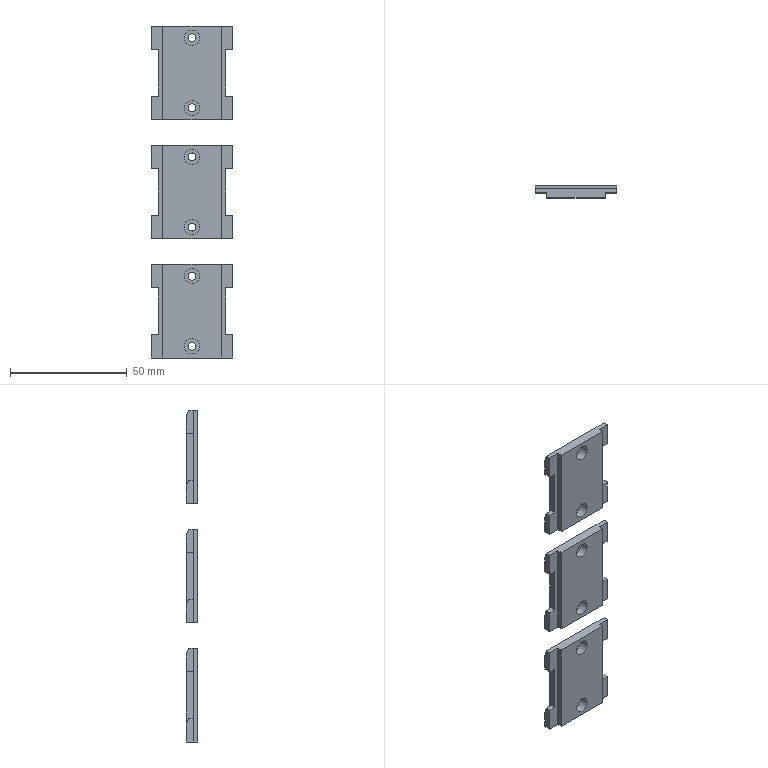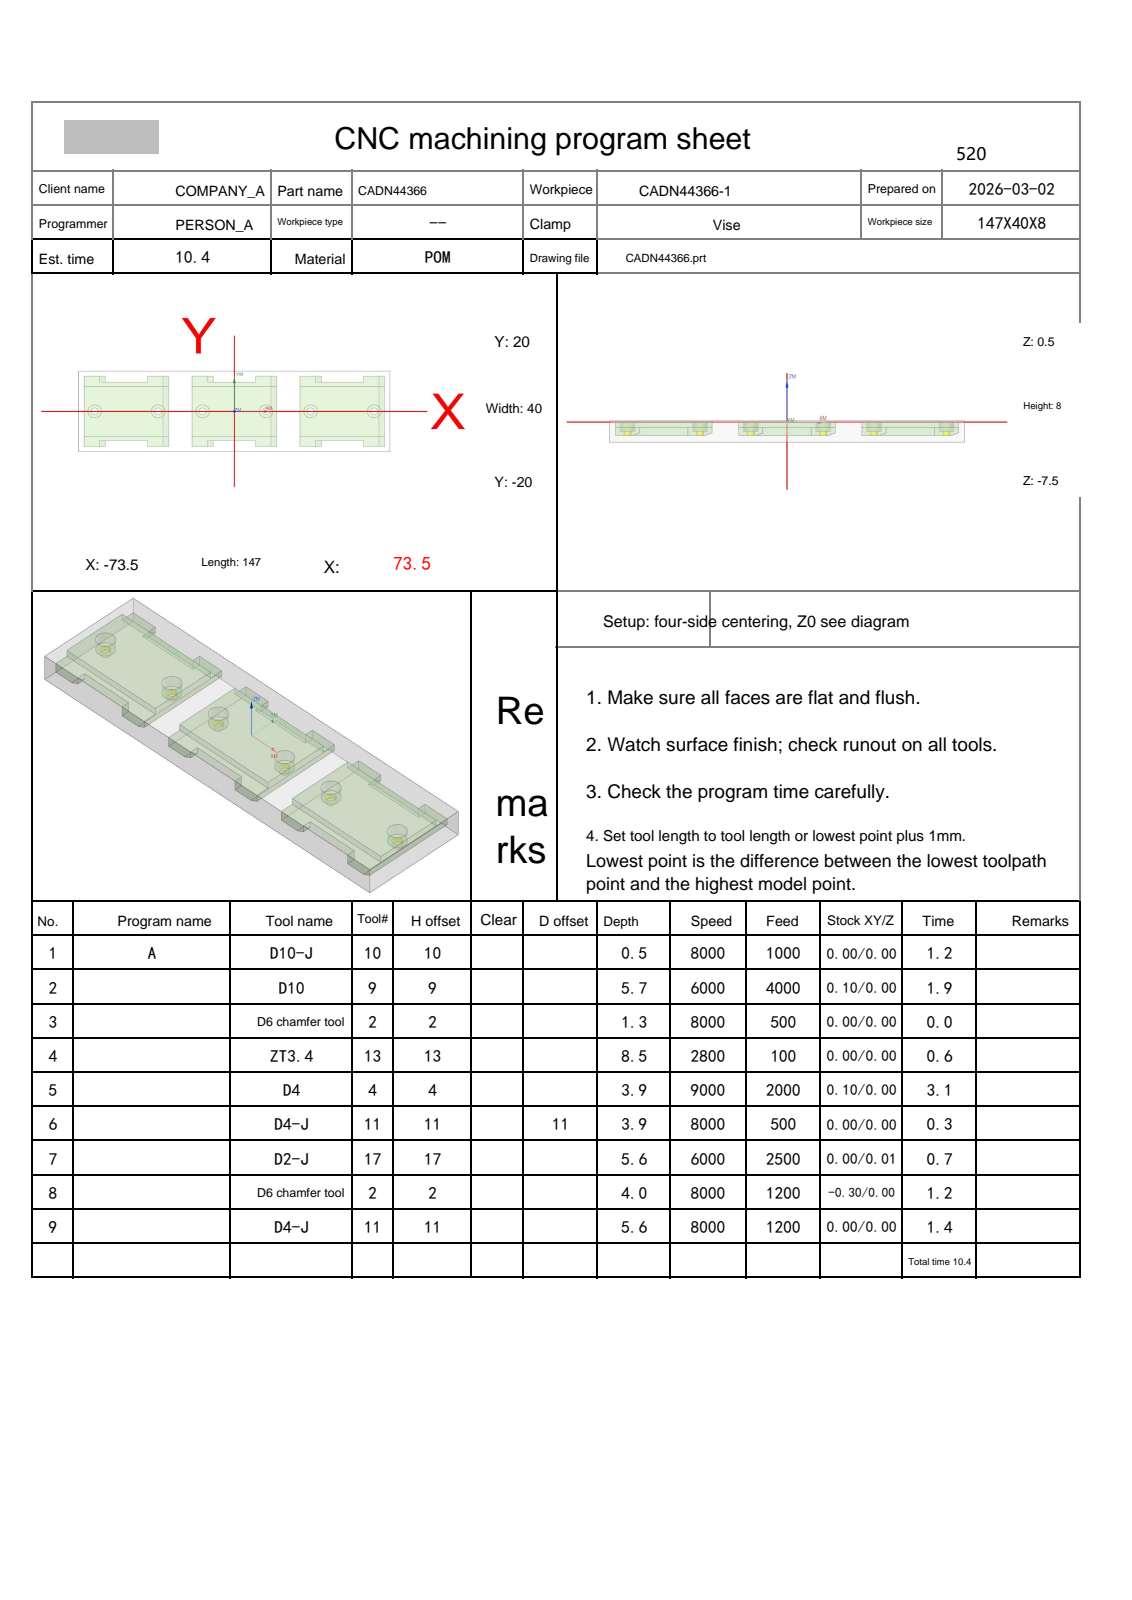NC program | NX | posted by the shop | part box 35 x 5 x 142 mm
Lines 1 to 1788 of 5584:
%
O0001
(Machine time: 11.93 MIN)
(===Total Tool:7===)
(T10=D10-J  D=10.  R=0.   D-  H10 Z=0.    )
(T9=D10     D=10.  R=0.   D-  H09 Z=-5.2  )
(T2=D6 chamfer tool   D=6.   R=0.   D-  H02 Z=-3.5  )
(T13=ZT3.4  D=3.4  DR_a=118 D-  H13 Z=-8.02 )
(T4=D4      D=4.   R=0.   D-  H04 Z=-3.4  )
(T11=D4-J   D=4.   R=0.   D11 H11 Z=-5.1  )
(T17=D2-J   D=2.   R=0.   D-  H17 Z=-5.1  )
G80 G90 G17 G49 G40
G91 G28 Z0
M01
N1 T10 M06
(D10-J  D=10. R=0. H=10 ce=0.00 di=0.00)
G00 G90 G54 X-88. Y.65 M03 S8000
G43 H10 Z30.
M08
Z2.
G01 Z0.0 F1000.
X-76. Y12.65
X-66.15 Y22.5
X-56.3
X-76. Y2.8
Y-7.05
X-46.45 Y22.5
X-36.6
X-76. Y-16.9
Y-22.5
X-71.75
X-26.75 Y22.5
X-16.9
X-61.9 Y-22.5
X-52.05
X-7.05 Y22.5
X2.8
X-42.2 Y-22.5
X-32.35
X12.65 Y22.5
X22.5
X-22.5 Y-22.5
X-12.65
X32.35 Y22.5
X42.2
X-2.8 Y-22.5
X7.05
X52.05 Y22.5
X61.9
X16.9 Y-22.5
X26.75
X71.75 Y22.5
X76.
Y16.9
X36.6 Y-22.5
X46.45
X76. Y7.05
Y-2.8
X56.3 Y-22.5
X66.15
X76. Y-12.65
X88. Y-.65
Z2.
G00 Z30.
G91 G28 Z0.0
M05
M09
G91 G28 Z0.0
M01
N2 T09 M06
(D10  D=10. R=0. H=09 ce=0.10 di=0.00)
G00 G90 G54 X76.1 Y0.0 M03 S6000
G43 H09 Z30.
M08
Z.5
G01 Y-17.5 Z.456 F4000.
G02 X71. Y-22.6 Z.435 I-5.1 J0.0
G01 X61. Z.41
G02 X56.352 Y-19.6 Z.395 I0.0 J5.1
G01 X45.648 Z.368
G02 X41. Y-22.6 Z.353 I-4.648 J2.1
G01 X31. Z.327
G02 X25.9 Y-17.5 Z.307 I0.0 J5.1
G01 Y17.5 Z.218
G02 X31. Y22.6 Z.198 I5.1 J0.0
G01 X41. Z.172
G02 X45.648 Y19.6 Z.157 I0.0 J-5.1
G01 X56.352 Z.13
G02 X61. Y22.6 Z.115 I4.648 J-2.1
G01 X71. Z.09
G02 X76.1 Y17.5 Z.069 I0.0 J-5.1
G01 Y-17.5 Z-.019
G02 X71. Y-22.6 Z-.04 I-5.1 J0.0
G01 X61. Z-.065
G02 X56.352 Y-19.6 Z-.08 I0.0 J5.1
G01 X45.648 Z-.107
G02 X41. Y-22.6 Z-.122 I-4.648 J2.1
G01 X31. Z-.148
G02 X25.9 Y-17.5 Z-.168 I0.0 J5.1
G01 Y17.5 Z-.257
G02 X31. Y22.6 Z-.277 I5.1 J0.0
G01 X41. Z-.303
G02 X45.648 Y19.6 Z-.318 I0.0 J-5.1
G01 X56.352 Z-.345
G02 X61. Y22.6 Z-.36 I4.648 J-2.1
G01 X71. Z-.385
G02 X76.1 Y17.5 Z-.406 I0.0 J-5.1
G01 Y-17.5 Z-.494
G02 X71. Y-22.6 Z-.515 I-5.1 J0.0
G01 X61. Z-.54
G02 X56.352 Y-19.6 Z-.555 I0.0 J5.1
G01 X45.648 Z-.582
G02 X41. Y-22.6 Z-.597 I-4.648 J2.1
G01 X31. Z-.623
G02 X25.9 Y-17.5 Z-.643 I0.0 J5.1
G01 Y17.5 Z-.732
G02 X31. Y22.6 Z-.752 I5.1 J0.0
G01 X41. Z-.778
G02 X45.648 Y19.6 Z-.793 I0.0 J-5.1
G01 X56.352 Z-.82
G02 X61. Y22.6 Z-.835 I4.648 J-2.1
G01 X71. Z-.86
G02 X76.1 Y17.5 Z-.881 I0.0 J-5.1
G01 Y-17.5 Z-.969
G02 X71. Y-22.6 Z-.99 I-5.1 J0.0
G01 X61. Z-1.015
G02 X56.352 Y-19.6 Z-1.03 I0.0 J5.1
G01 X45.648 Z-1.057
G02 X41. Y-22.6 Z-1.072 I-4.648 J2.1
G01 X31. Z-1.098
G02 X25.9 Y-17.5 Z-1.118 I0.0 J5.1
G01 Y17.5 Z-1.207
G02 X31. Y22.6 Z-1.227 I5.1 J0.0
G01 X41. Z-1.253
G02 X45.648 Y19.6 Z-1.268 I0.0 J-5.1
G01 X56.352 Z-1.295
G02 X61. Y22.6 Z-1.31 I4.648 J-2.1
G01 X71. Z-1.335
G02 X76.1 Y17.5 Z-1.356 I0.0 J-5.1
G01 Y-17.5 Z-1.444
G02 X71. Y-22.6 Z-1.465 I-5.1 J0.0
G01 X61. Z-1.49
G02 X56.352 Y-19.6 Z-1.505 I0.0 J5.1
G01 X45.648 Z-1.532
G02 X41. Y-22.6 Z-1.547 I-4.648 J2.1
G01 X31. Z-1.573
G02 X25.9 Y-17.5 Z-1.593 I0.0 J5.1
G01 Y17.5 Z-1.682
G02 X31. Y22.6 Z-1.702 I5.1 J0.0
G01 X41. Z-1.728
G02 X45.648 Y19.6 Z-1.743 I0.0 J-5.1
G01 X56.352 Z-1.77
G02 X61. Y22.6 Z-1.785 I4.648 J-2.1
G01 X71. Z-1.81
G02 X76.1 Y17.5 Z-1.831 I0.0 J-5.1
G01 Y-17.5 Z-1.919
G02 X71. Y-22.6 Z-1.94 I-5.1 J0.0
G01 X61. Z-1.965
G02 X56.352 Y-19.6 Z-1.98 I0.0 J5.1
G01 X45.648 Z-2.007
G02 X41. Y-22.6 Z-2.022 I-4.648 J2.1
G01 X31. Z-2.048
G02 X25.9 Y-17.5 Z-2.068 I0.0 J5.1
G01 Y17.5 Z-2.157
G02 X31. Y22.6 Z-2.177 I5.1 J0.0
G01 X41. Z-2.203
G02 X45.648 Y19.6 Z-2.218 I0.0 J-5.1
G01 X56.352 Z-2.245
G02 X61. Y22.6 Z-2.26 I4.648 J-2.1
G01 X71. Z-2.285
G02 X76.1 Y17.5 Z-2.306 I0.0 J-5.1
G01 Y-17.5 Z-2.394
G02 X71. Y-22.6 Z-2.415 I-5.1 J0.0
G01 X61. Z-2.44
G02 X56.352 Y-19.6 Z-2.455 I0.0 J5.1
G01 X45.648 Z-2.482
G02 X41. Y-22.6 Z-2.497 I-4.648 J2.1
G01 X31. Z-2.523
G02 X25.9 Y-17.5 Z-2.543 I0.0 J5.1
G01 Y17.5 Z-2.632
G02 X31. Y22.6 Z-2.652 I5.1 J0.0
G01 X41. Z-2.678
G02 X45.648 Y19.6 Z-2.693 I0.0 J-5.1
G01 X56.352 Z-2.72
G02 X61. Y22.6 Z-2.735 I4.648 J-2.1
G01 X71. Z-2.76
G02 X76.1 Y17.5 Z-2.781 I0.0 J-5.1
G01 Y-17.5 Z-2.869
G02 X71. Y-22.6 Z-2.89 I-5.1 J0.0
G01 X61. Z-2.915
G02 X56.352 Y-19.6 Z-2.93 I0.0 J5.1
G01 X45.648 Z-2.957
G02 X41. Y-22.6 Z-2.972 I-4.648 J2.1
G01 X31. Z-2.998
G02 X25.9 Y-17.5 Z-3.018 I0.0 J5.1
G01 Y17.5 Z-3.107
G02 X31. Y22.6 Z-3.127 I5.1 J0.0
G01 X41. Z-3.153
G02 X45.648 Y19.6 Z-3.168 I0.0 J-5.1
G01 X56.352 Z-3.195
G02 X61. Y22.6 Z-3.21 I4.648 J-2.1
G01 X71. Z-3.235
G02 X76.1 Y17.5 Z-3.256 I0.0 J-5.1
G01 Y-17.5 Z-3.344
G02 X71. Y-22.6 Z-3.365 I-5.1 J0.0
G01 X61. Z-3.39
G02 X56.352 Y-19.6 Z-3.405 I0.0 J5.1
G01 X45.648 Z-3.432
G02 X41. Y-22.6 Z-3.447 I-4.648 J2.1
G01 X31. Z-3.473
G02 X25.9 Y-17.5 Z-3.493 I0.0 J5.1
G01 Y17.5 Z-3.582
G02 X31. Y22.6 Z-3.602 I5.1 J0.0
G01 X41. Z-3.628
G02 X45.648 Y19.6 Z-3.643 I0.0 J-5.1
G01 X56.352 Z-3.67
G02 X61. Y22.6 Z-3.685 I4.648 J-2.1
G01 X71. Z-3.71
G02 X76.1 Y17.5 Z-3.731 I0.0 J-5.1
G01 Y-17.5 Z-3.819
G02 X71. Y-22.6 Z-3.84 I-5.1 J0.0
G01 X61. Z-3.865
G02 X56.352 Y-19.6 Z-3.88 I0.0 J5.1
G01 X45.648 Z-3.907
G02 X41. Y-22.6 Z-3.922 I-4.648 J2.1
G01 X31. Z-3.948
G02 X25.9 Y-17.5 Z-3.968 I0.0 J5.1
G01 Y17.5 Z-4.057
G02 X31. Y22.6 Z-4.077 I5.1 J0.0
G01 X41. Z-4.103
G02 X45.648 Y19.6 Z-4.118 I0.0 J-5.1
G01 X56.352 Z-4.145
G02 X61. Y22.6 Z-4.16 I4.648 J-2.1
G01 X71. Z-4.185
G02 X76.1 Y17.5 Z-4.206 I0.0 J-5.1
G01 Y-17.5 Z-4.294
G02 X71. Y-22.6 Z-4.315 I-5.1 J0.0
G01 X61. Z-4.34
G02 X56.352 Y-19.6 Z-4.355 I0.0 J5.1
G01 X45.648 Z-4.382
G02 X41. Y-22.6 Z-4.397 I-4.648 J2.1
G01 X31. Z-4.423
G02 X25.9 Y-17.5 Z-4.443 I0.0 J5.1
G01 Y17.5 Z-4.532
G02 X31. Y22.6 Z-4.552 I5.1 J0.0
G01 X41. Z-4.578
G02 X45.648 Y19.6 Z-4.593 I0.0 J-5.1
G01 X56.352 Z-4.62
G02 X61. Y22.6 Z-4.635 I4.648 J-2.1
G01 X71. Z-4.66
G02 X76.1 Y17.5 Z-4.681 I0.0 J-5.1
G01 Y-17.5 Z-4.769
G02 X71. Y-22.6 Z-4.79 I-5.1 J0.0
G01 X61. Z-4.815
G02 X56.352 Y-19.6 Z-4.83 I0.0 J5.1
G01 X45.648 Z-4.857
G02 X41. Y-22.6 Z-4.872 I-4.648 J2.1
G01 X31. Z-4.898
G02 X25.9 Y-17.5 Z-4.918 I0.0 J5.1
G01 Y17.5 Z-5.007
G02 X31. Y22.6 Z-5.027 I5.1 J0.0
G01 X41. Z-5.053
G02 X45.648 Y19.6 Z-5.068 I0.0 J-5.1
G01 X56.352 Z-5.095
G02 X61. Y22.6 Z-5.11 I4.648 J-2.1
G01 X71. Z-5.135
G02 X76.1 Y17.5 Z-5.156 I0.0 J-5.1
G01 Y0.0 Z-5.2
Y-17.5
G02 X71. Y-22.6 I-5.1 J0.0
G01 X61.
G02 X56.352 Y-19.6 I0.0 J5.1
G01 X45.648
G02 X41. Y-22.6 I-4.648 J2.1
G01 X31.
G02 X25.9 Y-17.5 I0.0 J5.1
G01 Y17.5
G02 X31. Y22.6 I5.1 J0.0
G01 X41.
G02 X45.648 Y19.6 I0.0 J-5.1
G01 X56.352
G02 X61. Y22.6 I4.648 J-2.1
G01 X71.
G02 X76.1 Y17.5 I0.0 J-5.1
G01 Y0.0
Y-.5
Z-4.2
G00 Z30.
X25.1 Y0.0
Z.5
G01 Y-17.5 Z.456
G02 X20. Y-22.6 Z.435 I-5.1 J0.0
G01 X10. Z.41
G02 X5.352 Y-19.6 Z.395 I0.0 J5.1
G01 X-5.352 Z.368
G02 X-10. Y-22.6 Z.353 I-4.648 J2.1
G01 X-20. Z.327
G02 X-25.1 Y-17.5 Z.307 I0.0 J5.1
G01 Y17.5 Z.218
G02 X-20. Y22.6 Z.198 I5.1 J0.0
G01 X-10. Z.172
G02 X-5.352 Y19.6 Z.157 I0.0 J-5.1
G01 X5.352 Z.13
G02 X10. Y22.6 Z.115 I4.648 J-2.1
G01 X20. Z.09
G02 X25.1 Y17.5 Z.069 I0.0 J-5.1
G01 Y-17.5 Z-.019
G02 X20. Y-22.6 Z-.04 I-5.1 J0.0
G01 X10. Z-.065
G02 X5.352 Y-19.6 Z-.08 I0.0 J5.1
G01 X-5.352 Z-.107
G02 X-10. Y-22.6 Z-.122 I-4.648 J2.1
G01 X-20. Z-.148
G02 X-25.1 Y-17.5 Z-.168 I0.0 J5.1
G01 Y17.5 Z-.257
G02 X-20. Y22.6 Z-.277 I5.1 J0.0
G01 X-10. Z-.303
G02 X-5.352 Y19.6 Z-.318 I0.0 J-5.1
G01 X5.352 Z-.345
G02 X10. Y22.6 Z-.36 I4.648 J-2.1
G01 X20. Z-.385
G02 X25.1 Y17.5 Z-.406 I0.0 J-5.1
G01 Y-17.5 Z-.494
G02 X20. Y-22.6 Z-.515 I-5.1 J0.0
G01 X10. Z-.54
G02 X5.352 Y-19.6 Z-.555 I0.0 J5.1
G01 X-5.352 Z-.582
G02 X-10. Y-22.6 Z-.597 I-4.648 J2.1
G01 X-20. Z-.623
G02 X-25.1 Y-17.5 Z-.643 I0.0 J5.1
G01 Y17.5 Z-.732
G02 X-20. Y22.6 Z-.752 I5.1 J0.0
G01 X-10. Z-.778
G02 X-5.352 Y19.6 Z-.793 I0.0 J-5.1
G01 X5.352 Z-.82
G02 X10. Y22.6 Z-.835 I4.648 J-2.1
G01 X20. Z-.86
G02 X25.1 Y17.5 Z-.881 I0.0 J-5.1
G01 Y-17.5 Z-.969
G02 X20. Y-22.6 Z-.99 I-5.1 J0.0
G01 X10. Z-1.015
G02 X5.352 Y-19.6 Z-1.03 I0.0 J5.1
G01 X-5.352 Z-1.057
G02 X-10. Y-22.6 Z-1.072 I-4.648 J2.1
G01 X-20. Z-1.098
G02 X-25.1 Y-17.5 Z-1.118 I0.0 J5.1
G01 Y17.5 Z-1.207
G02 X-20. Y22.6 Z-1.227 I5.1 J0.0
G01 X-10. Z-1.253
G02 X-5.352 Y19.6 Z-1.268 I0.0 J-5.1
G01 X5.352 Z-1.295
G02 X10. Y22.6 Z-1.31 I4.648 J-2.1
G01 X20. Z-1.335
G02 X25.1 Y17.5 Z-1.356 I0.0 J-5.1
G01 Y-17.5 Z-1.444
G02 X20. Y-22.6 Z-1.465 I-5.1 J0.0
G01 X10. Z-1.49
G02 X5.352 Y-19.6 Z-1.505 I0.0 J5.1
G01 X-5.352 Z-1.532
G02 X-10. Y-22.6 Z-1.547 I-4.648 J2.1
G01 X-20. Z-1.573
G02 X-25.1 Y-17.5 Z-1.593 I0.0 J5.1
G01 Y17.5 Z-1.682
G02 X-20. Y22.6 Z-1.702 I5.1 J0.0
G01 X-10. Z-1.728
G02 X-5.352 Y19.6 Z-1.743 I0.0 J-5.1
G01 X5.352 Z-1.77
G02 X10. Y22.6 Z-1.785 I4.648 J-2.1
G01 X20. Z-1.81
G02 X25.1 Y17.5 Z-1.831 I0.0 J-5.1
G01 Y-17.5 Z-1.919
G02 X20. Y-22.6 Z-1.94 I-5.1 J0.0
G01 X10. Z-1.965
G02 X5.352 Y-19.6 Z-1.98 I0.0 J5.1
G01 X-5.352 Z-2.007
G02 X-10. Y-22.6 Z-2.022 I-4.648 J2.1
G01 X-20. Z-2.048
G02 X-25.1 Y-17.5 Z-2.068 I0.0 J5.1
G01 Y17.5 Z-2.157
G02 X-20. Y22.6 Z-2.177 I5.1 J0.0
G01 X-10. Z-2.203
G02 X-5.352 Y19.6 Z-2.218 I0.0 J-5.1
G01 X5.352 Z-2.245
G02 X10. Y22.6 Z-2.26 I4.648 J-2.1
G01 X20. Z-2.285
G02 X25.1 Y17.5 Z-2.306 I0.0 J-5.1
G01 Y-17.5 Z-2.394
G02 X20. Y-22.6 Z-2.415 I-5.1 J0.0
G01 X10. Z-2.44
G02 X5.352 Y-19.6 Z-2.455 I0.0 J5.1
G01 X-5.352 Z-2.482
G02 X-10. Y-22.6 Z-2.497 I-4.648 J2.1
G01 X-20. Z-2.523
G02 X-25.1 Y-17.5 Z-2.543 I0.0 J5.1
G01 Y17.5 Z-2.632
G02 X-20. Y22.6 Z-2.652 I5.1 J0.0
G01 X-10. Z-2.678
G02 X-5.352 Y19.6 Z-2.693 I0.0 J-5.1
G01 X5.352 Z-2.72
G02 X10. Y22.6 Z-2.735 I4.648 J-2.1
G01 X20. Z-2.76
G02 X25.1 Y17.5 Z-2.781 I0.0 J-5.1
G01 Y-17.5 Z-2.869
G02 X20. Y-22.6 Z-2.89 I-5.1 J0.0
G01 X10. Z-2.915
G02 X5.352 Y-19.6 Z-2.93 I0.0 J5.1
G01 X-5.352 Z-2.957
G02 X-10. Y-22.6 Z-2.972 I-4.648 J2.1
G01 X-20. Z-2.998
G02 X-25.1 Y-17.5 Z-3.018 I0.0 J5.1
G01 Y17.5 Z-3.107
G02 X-20. Y22.6 Z-3.127 I5.1 J0.0
G01 X-10. Z-3.153
G02 X-5.352 Y19.6 Z-3.168 I0.0 J-5.1
G01 X5.352 Z-3.195
G02 X10. Y22.6 Z-3.21 I4.648 J-2.1
G01 X20. Z-3.235
G02 X25.1 Y17.5 Z-3.256 I0.0 J-5.1
G01 Y-17.5 Z-3.344
G02 X20. Y-22.6 Z-3.365 I-5.1 J0.0
G01 X10. Z-3.39
G02 X5.352 Y-19.6 Z-3.405 I0.0 J5.1
G01 X-5.352 Z-3.432
G02 X-10. Y-22.6 Z-3.447 I-4.648 J2.1
G01 X-20. Z-3.473
G02 X-25.1 Y-17.5 Z-3.493 I0.0 J5.1
G01 Y17.5 Z-3.582
G02 X-20. Y22.6 Z-3.602 I5.1 J0.0
G01 X-10. Z-3.628
G02 X-5.352 Y19.6 Z-3.643 I0.0 J-5.1
G01 X5.352 Z-3.67
G02 X10. Y22.6 Z-3.685 I4.648 J-2.1
G01 X20. Z-3.71
G02 X25.1 Y17.5 Z-3.731 I0.0 J-5.1
G01 Y-17.5 Z-3.819
G02 X20. Y-22.6 Z-3.84 I-5.1 J0.0
G01 X10. Z-3.865
G02 X5.352 Y-19.6 Z-3.88 I0.0 J5.1
G01 X-5.352 Z-3.907
G02 X-10. Y-22.6 Z-3.922 I-4.648 J2.1
G01 X-20. Z-3.948
G02 X-25.1 Y-17.5 Z-3.968 I0.0 J5.1
G01 Y17.5 Z-4.057
G02 X-20. Y22.6 Z-4.077 I5.1 J0.0
G01 X-10. Z-4.103
G02 X-5.352 Y19.6 Z-4.118 I0.0 J-5.1
G01 X5.352 Z-4.145
G02 X10. Y22.6 Z-4.16 I4.648 J-2.1
G01 X20. Z-4.185
G02 X25.1 Y17.5 Z-4.206 I0.0 J-5.1
G01 Y-17.5 Z-4.294
G02 X20. Y-22.6 Z-4.315 I-5.1 J0.0
G01 X10. Z-4.34
G02 X5.352 Y-19.6 Z-4.355 I0.0 J5.1
G01 X-5.352 Z-4.382
G02 X-10. Y-22.6 Z-4.397 I-4.648 J2.1
G01 X-20. Z-4.423
G02 X-25.1 Y-17.5 Z-4.443 I0.0 J5.1
G01 Y17.5 Z-4.532
G02 X-20. Y22.6 Z-4.552 I5.1 J0.0
G01 X-10. Z-4.578
G02 X-5.352 Y19.6 Z-4.593 I0.0 J-5.1
G01 X5.352 Z-4.62
G02 X10. Y22.6 Z-4.635 I4.648 J-2.1
G01 X20. Z-4.66
G02 X25.1 Y17.5 Z-4.681 I0.0 J-5.1
G01 Y-17.5 Z-4.769
G02 X20. Y-22.6 Z-4.79 I-5.1 J0.0
G01 X10. Z-4.815
G02 X5.352 Y-19.6 Z-4.83 I0.0 J5.1
G01 X-5.352 Z-4.857
G02 X-10. Y-22.6 Z-4.872 I-4.648 J2.1
G01 X-20. Z-4.898
G02 X-25.1 Y-17.5 Z-4.918 I0.0 J5.1
G01 Y17.5 Z-5.007
G02 X-20. Y22.6 Z-5.027 I5.1 J0.0
G01 X-10. Z-5.053
G02 X-5.352 Y19.6 Z-5.068 I0.0 J-5.1
G01 X5.352 Z-5.095
G02 X10. Y22.6 Z-5.11 I4.648 J-2.1
G01 X20. Z-5.135
G02 X25.1 Y17.5 Z-5.156 I0.0 J-5.1
G01 Y0.0 Z-5.2
Y-17.5
G02 X20. Y-22.6 I-5.1 J0.0
G01 X10.
G02 X5.352 Y-19.6 I0.0 J5.1
G01 X-5.352
G02 X-10. Y-22.6 I-4.648 J2.1
G01 X-20.
G02 X-25.1 Y-17.5 I0.0 J5.1
G01 Y17.5
G02 X-20. Y22.6 I5.1 J0.0
G01 X-10.
G02 X-5.352 Y19.6 I0.0 J-5.1
G01 X5.352
G02 X10. Y22.6 I4.648 J-2.1
G01 X20.
G02 X25.1 Y17.5 I0.0 J-5.1
G01 Y0.0
Y-.5
Z-4.2
G00 Z30.
X-76.1 Y0.0
Z.5
G01 Y17.5 Z.456
G02 X-71. Y22.6 Z.435 I5.1 J0.0
G01 X-61. Z.41
G02 X-56.352 Y19.6 Z.395 I0.0 J-5.1
G01 X-45.648 Z.368
G02 X-41. Y22.6 Z.353 I4.648 J-2.1
G01 X-31. Z.327
G02 X-25.9 Y17.5 Z.307 I0.0 J-5.1
G01 Y-17.5 Z.218
G02 X-31. Y-22.6 Z.198 I-5.1 J0.0
G01 X-41. Z.172
G02 X-45.648 Y-19.6 Z.157 I0.0 J5.1
G01 X-56.352 Z.13
G02 X-61. Y-22.6 Z.115 I-4.648 J2.1
G01 X-71. Z.09
G02 X-76.1 Y-17.5 Z.069 I0.0 J5.1
G01 Y17.5 Z-.019
G02 X-71. Y22.6 Z-.04 I5.1 J0.0
G01 X-61. Z-.065
G02 X-56.352 Y19.6 Z-.08 I0.0 J-5.1
G01 X-45.648 Z-.107
G02 X-41. Y22.6 Z-.122 I4.648 J-2.1
G01 X-31. Z-.148
G02 X-25.9 Y17.5 Z-.168 I0.0 J-5.1
G01 Y-17.5 Z-.257
G02 X-31. Y-22.6 Z-.277 I-5.1 J0.0
G01 X-41. Z-.303
G02 X-45.648 Y-19.6 Z-.318 I0.0 J5.1
G01 X-56.352 Z-.345
G02 X-61. Y-22.6 Z-.36 I-4.648 J2.1
G01 X-71. Z-.385
G02 X-76.1 Y-17.5 Z-.406 I0.0 J5.1
G01 Y17.5 Z-.494
G02 X-71. Y22.6 Z-.515 I5.1 J0.0
G01 X-61. Z-.54
G02 X-56.352 Y19.6 Z-.555 I0.0 J-5.1
G01 X-45.648 Z-.582
G02 X-41. Y22.6 Z-.597 I4.648 J-2.1
G01 X-31. Z-.623
G02 X-25.9 Y17.5 Z-.643 I0.0 J-5.1
G01 Y-17.5 Z-.732
G02 X-31. Y-22.6 Z-.752 I-5.1 J0.0
G01 X-41. Z-.778
G02 X-45.648 Y-19.6 Z-.793 I0.0 J5.1
G01 X-56.352 Z-.82
G02 X-61. Y-22.6 Z-.835 I-4.648 J2.1
G01 X-71. Z-.86
G02 X-76.1 Y-17.5 Z-.881 I0.0 J5.1
G01 Y17.5 Z-.969
G02 X-71. Y22.6 Z-.99 I5.1 J0.0
G01 X-61. Z-1.015
G02 X-56.352 Y19.6 Z-1.03 I0.0 J-5.1
G01 X-45.648 Z-1.057
G02 X-41. Y22.6 Z-1.072 I4.648 J-2.1
G01 X-31. Z-1.098
G02 X-25.9 Y17.5 Z-1.118 I0.0 J-5.1
G01 Y-17.5 Z-1.207
G02 X-31. Y-22.6 Z-1.227 I-5.1 J0.0
G01 X-41. Z-1.253
G02 X-45.648 Y-19.6 Z-1.268 I0.0 J5.1
G01 X-56.352 Z-1.295
G02 X-61. Y-22.6 Z-1.31 I-4.648 J2.1
G01 X-71. Z-1.335
G02 X-76.1 Y-17.5 Z-1.356 I0.0 J5.1
G01 Y17.5 Z-1.444
G02 X-71. Y22.6 Z-1.465 I5.1 J0.0
G01 X-61. Z-1.49
G02 X-56.352 Y19.6 Z-1.505 I0.0 J-5.1
G01 X-45.648 Z-1.532
G02 X-41. Y22.6 Z-1.547 I4.648 J-2.1
G01 X-31. Z-1.573
G02 X-25.9 Y17.5 Z-1.593 I0.0 J-5.1
G01 Y-17.5 Z-1.682
G02 X-31. Y-22.6 Z-1.702 I-5.1 J0.0
G01 X-41. Z-1.728
G02 X-45.648 Y-19.6 Z-1.743 I0.0 J5.1
G01 X-56.352 Z-1.77
G02 X-61. Y-22.6 Z-1.785 I-4.648 J2.1
G01 X-71. Z-1.81
G02 X-76.1 Y-17.5 Z-1.831 I0.0 J5.1
G01 Y17.5 Z-1.919
G02 X-71. Y22.6 Z-1.94 I5.1 J0.0
G01 X-61. Z-1.965
G02 X-56.352 Y19.6 Z-1.98 I0.0 J-5.1
G01 X-45.648 Z-2.007
G02 X-41. Y22.6 Z-2.022 I4.648 J-2.1
G01 X-31. Z-2.048
G02 X-25.9 Y17.5 Z-2.068 I0.0 J-5.1
G01 Y-17.5 Z-2.157
G02 X-31. Y-22.6 Z-2.177 I-5.1 J0.0
G01 X-41. Z-2.203
G02 X-45.648 Y-19.6 Z-2.218 I0.0 J5.1
G01 X-56.352 Z-2.245
G02 X-61. Y-22.6 Z-2.26 I-4.648 J2.1
G01 X-71. Z-2.285
G02 X-76.1 Y-17.5 Z-2.306 I0.0 J5.1
G01 Y17.5 Z-2.394
G02 X-71. Y22.6 Z-2.415 I5.1 J0.0
G01 X-61. Z-2.44
G02 X-56.352 Y19.6 Z-2.455 I0.0 J-5.1
G01 X-45.648 Z-2.482
G02 X-41. Y22.6 Z-2.497 I4.648 J-2.1
G01 X-31. Z-2.523
G02 X-25.9 Y17.5 Z-2.543 I0.0 J-5.1
G01 Y-17.5 Z-2.632
G02 X-31. Y-22.6 Z-2.652 I-5.1 J0.0
G01 X-41. Z-2.678
G02 X-45.648 Y-19.6 Z-2.693 I0.0 J5.1
G01 X-56.352 Z-2.72
G02 X-61. Y-22.6 Z-2.735 I-4.648 J2.1
G01 X-71. Z-2.76
G02 X-76.1 Y-17.5 Z-2.781 I0.0 J5.1
G01 Y17.5 Z-2.869
G02 X-71. Y22.6 Z-2.89 I5.1 J0.0
G01 X-61. Z-2.915
G02 X-56.352 Y19.6 Z-2.93 I0.0 J-5.1
G01 X-45.648 Z-2.957
G02 X-41. Y22.6 Z-2.972 I4.648 J-2.1
G01 X-31. Z-2.998
G02 X-25.9 Y17.5 Z-3.018 I0.0 J-5.1
G01 Y-17.5 Z-3.107
G02 X-31. Y-22.6 Z-3.127 I-5.1 J0.0
G01 X-41. Z-3.153
G02 X-45.648 Y-19.6 Z-3.168 I0.0 J5.1
G01 X-56.352 Z-3.195
G02 X-61. Y-22.6 Z-3.21 I-4.648 J2.1
G01 X-71. Z-3.235
G02 X-76.1 Y-17.5 Z-3.256 I0.0 J5.1
G01 Y17.5 Z-3.344
G02 X-71. Y22.6 Z-3.365 I5.1 J0.0
G01 X-61. Z-3.39
G02 X-56.352 Y19.6 Z-3.405 I0.0 J-5.1
G01 X-45.648 Z-3.432
G02 X-41. Y22.6 Z-3.447 I4.648 J-2.1
G01 X-31. Z-3.473
G02 X-25.9 Y17.5 Z-3.493 I0.0 J-5.1
G01 Y-17.5 Z-3.582
G02 X-31. Y-22.6 Z-3.602 I-5.1 J0.0
G01 X-41. Z-3.628
G02 X-45.648 Y-19.6 Z-3.643 I0.0 J5.1
G01 X-56.352 Z-3.67
G02 X-61. Y-22.6 Z-3.685 I-4.648 J2.1
G01 X-71. Z-3.71
G02 X-76.1 Y-17.5 Z-3.731 I0.0 J5.1
G01 Y17.5 Z-3.819
G02 X-71. Y22.6 Z-3.84 I5.1 J0.0
G01 X-61. Z-3.865
G02 X-56.352 Y19.6 Z-3.88 I0.0 J-5.1
G01 X-45.648 Z-3.907
G02 X-41. Y22.6 Z-3.922 I4.648 J-2.1
G01 X-31. Z-3.948
G02 X-25.9 Y17.5 Z-3.968 I0.0 J-5.1
G01 Y-17.5 Z-4.057
G02 X-31. Y-22.6 Z-4.077 I-5.1 J0.0
G01 X-41. Z-4.103
G02 X-45.648 Y-19.6 Z-4.118 I0.0 J5.1
G01 X-56.352 Z-4.145
G02 X-61. Y-22.6 Z-4.16 I-4.648 J2.1
G01 X-71. Z-4.185
G02 X-76.1 Y-17.5 Z-4.206 I0.0 J5.1
G01 Y17.5 Z-4.294
G02 X-71. Y22.6 Z-4.315 I5.1 J0.0
G01 X-61. Z-4.34
G02 X-56.352 Y19.6 Z-4.355 I0.0 J-5.1
G01 X-45.648 Z-4.382
G02 X-41. Y22.6 Z-4.397 I4.648 J-2.1
G01 X-31. Z-4.423
G02 X-25.9 Y17.5 Z-4.443 I0.0 J-5.1
G01 Y-17.5 Z-4.532
G02 X-31. Y-22.6 Z-4.552 I-5.1 J0.0
G01 X-41. Z-4.578
G02 X-45.648 Y-19.6 Z-4.593 I0.0 J5.1
G01 X-56.352 Z-4.62
G02 X-61. Y-22.6 Z-4.635 I-4.648 J2.1
G01 X-71. Z-4.66
G02 X-76.1 Y-17.5 Z-4.681 I0.0 J5.1
G01 Y17.5 Z-4.769
G02 X-71. Y22.6 Z-4.79 I5.1 J0.0
G01 X-61. Z-4.815
G02 X-56.352 Y19.6 Z-4.83 I0.0 J-5.1
G01 X-45.648 Z-4.857
G02 X-41. Y22.6 Z-4.872 I4.648 J-2.1
G01 X-31. Z-4.898
G02 X-25.9 Y17.5 Z-4.918 I0.0 J-5.1
G01 Y-17.5 Z-5.007
G02 X-31. Y-22.6 Z-5.027 I-5.1 J0.0
G01 X-41. Z-5.053
G02 X-45.648 Y-19.6 Z-5.068 I0.0 J5.1
G01 X-56.352 Z-5.095
G02 X-61. Y-22.6 Z-5.11 I-4.648 J2.1
G01 X-71. Z-5.135
G02 X-76.1 Y-17.5 Z-5.156 I0.0 J5.1
G01 Y0.0 Z-5.2
Y17.5
G02 X-71. Y22.6 I5.1 J0.0
G01 X-61.
G02 X-56.352 Y19.6 I0.0 J-5.1
G01 X-45.648
G02 X-41. Y22.6 I4.648 J-2.1
G01 X-31.
G02 X-25.9 Y17.5 I0.0 J-5.1
G01 Y-17.5
G02 X-31. Y-22.6 I-5.1 J0.0
G01 X-41.
G02 X-45.648 Y-19.6 I0.0 J5.1
G01 X-56.352
G02 X-61. Y-22.6 I-4.648 J2.1
G01 X-71.
G02 X-76.1 Y-17.5 I0.0 J5.1
G01 Y0.0
Y.5
Z-4.2
G00 Z30.
G91 G28 Z0.0
M05
M09
G91 G28 Z0.0
M01
N3 T02 M06
(D6 chamfer tool  D=6. R=0. H=02 ce=0.00 di=0.00)
G00 G90 G54 X-66. Y0.0 M03 S8000
G43 H02 Z30.
M08
G98 G81 X-66. Y0.0 Z-.8 R1. F500.
X-36.
X-15.
X15.
X36.
X66.
G80
G00 Z30.
G91 G28 Z0.0
M05
M09
G91 G28 Z0.0
M01
N4 T13 M06
(ZT3.4 D=3.4 DR_a=118 H=13)
G00 G90 G54 X-66. Y0.0 M03 S2800
G43 H13 Z30.
M08
G98 G83 X-66. Y0.0 Z-8.021 R1. F100. Q2.
X-36.
X-15.
X15.
X36.
X66.
G80
G00 Z30.
G91 G28 Z0.0
M05
M09
G91 G28 Z0.0
M01
N5 T04 M06
(D4  D=4. R=0. H=04 ce=0.10 di=0.10)
G00 G90 G54 X51. Y19.5 M03 S9000
G43 H04 Z30.
M08
Z.263
G01 Z-.238 F2000.
Y14.9
X41.4
Y17.9
X30.6
Y14.6
X71.4
Y17.9
X60.6
Y14.9
X51.
X50.5
Z.263
G00 Z.5
X51. Y19.5
Z.025
G01 Z-.475
Y14.9
X41.4
Y17.9
X30.6
Y14.6
X71.4
Y17.9
X60.6
Y14.9
X51.
X50.5
Z.025
G00 Z.263
X51. Y19.5
Z-.213
G01 Z-.713
Y14.9
X41.4
Y17.9
X30.6
Y14.6
X71.4
Y17.9
X60.6
Y14.9
X51.
X50.5
Z-.213
G00 Z.025
X51. Y19.5
Z-.45
G01 Z-.95
Y14.9
X41.4
Y17.9
X30.6
Y14.6
X71.4
Y17.9
X60.6
Y14.9
X51.
X50.5
Z-.45
G00 Z-.213
X51. Y19.5
Z-.688
G01 Z-1.188
Y14.9
X41.4
Y17.9
X30.6
Y14.6
X71.4
Y17.9
X60.6
Y14.9
X51.
X50.5
Z-.688
G00 Z-.45
X51. Y19.5
Z-.925
G01 Z-1.425
Y14.9
X41.4
Y17.9
X30.6
Y14.6
X71.4
Y17.9
X60.6
Y14.9
X51.
X50.5
Z-.925
G00 Z-.688
X51. Y19.5
Z-1.163
G01 Z-1.663
Y14.9
X41.4
Y17.9
X30.6
Y14.6
X71.4
Y17.9
X60.6
Y14.9
X51.
X50.5
Z-1.163
G00 Z-.925
X51. Y19.5
Z-1.4
G01 Z-1.9
Y14.9
X41.4
Y17.9
X30.6
Y14.6
X71.4
Y17.9
X60.6
Y14.9
X51.
X50.5
Z-1.4
G00 Z30.
X51. Y-19.5
Z.263
G01 Z-.238
Y-14.9
X60.6
Y-17.9
X71.4
Y-14.6
X30.6
Y-17.9
X41.4
Y-14.9
X51.
X51.5
Z.263
G00 Z.5
X51. Y-19.5
Z.025
G01 Z-.475
Y-14.9
X60.6
Y-17.9
X71.4
Y-14.6
X30.6
Y-17.9
X41.4
Y-14.9
X51.
X51.5
Z.025
G00 Z.263
X51. Y-19.5
Z-.213
G01 Z-.713
Y-14.9
X60.6
Y-17.9
X71.4
Y-14.6
X30.6
Y-17.9
X41.4
Y-14.9
X51.
X51.5
Z-.213
G00 Z.025
X51. Y-19.5
Z-.45
G01 Z-.95
Y-14.9
X60.6
Y-17.9
X71.4
Y-14.6
X30.6
Y-17.9
X41.4
Y-14.9
X51.
X51.5
Z-.45
G00 Z-.213
X51. Y-19.5
Z-.688
G01 Z-1.188
Y-14.9
X60.6
Y-17.9
X71.4
Y-14.6
X30.6
Y-17.9
X41.4
Y-14.9
X51.
X51.5
Z-.688
G00 Z-.45
X51. Y-19.5
Z-.925
G01 Z-1.425
Y-14.9
X60.6
Y-17.9
X71.4
Y-14.6
X30.6
Y-17.9
X41.4
Y-14.9
X51.
X51.5
Z-.925
G00 Z-.688
X51. Y-19.5
Z-1.163
G01 Z-1.663
Y-14.9
X60.6
Y-17.9
X71.4
Y-14.6
X30.6
Y-17.9
X41.4
Y-14.9
X51.
X51.5
Z-1.163
G00 Z-.925
X51. Y-19.5
Z-1.4
G01 Z-1.9
Y-14.9
X60.6
Y-17.9
X71.4
Y-14.6
X30.6
Y-17.9
X41.4
Y-14.9
X51.
X51.5
Z-1.4
G00 Z30.
X0.0 Y-19.5
Z.263
G01 Z-.238
Y-14.9
X9.6
Y-17.9
X20.4
Y-14.6
X-20.4
Y-17.9
X-9.6
Y-14.9
X0.0
X.5
Z.263
G00 Z.5
X0.0 Y-19.5
Z.025
G01 Z-.475
Y-14.9
X9.6
Y-17.9
X20.4
Y-14.6
X-20.4
Y-17.9
X-9.6
Y-14.9
X0.0
X.5
Z.025
G00 Z.263
X0.0 Y-19.5
Z-.213
G01 Z-.713
Y-14.9
X9.6
Y-17.9
X20.4
Y-14.6
X-20.4
Y-17.9
X-9.6
Y-14.9
X0.0
X.5
Z-.213
G00 Z.025
X0.0 Y-19.5
Z-.45
G01 Z-.95
Y-14.9
X9.6
Y-17.9
X20.4
Y-14.6
X-20.4
Y-17.9
X-9.6
Y-14.9
X0.0
X.5
Z-.45
G00 Z-.213
X0.0 Y-19.5
Z-.688
G01 Z-1.188
Y-14.9
X9.6
Y-17.9
X20.4
Y-14.6
X-20.4
Y-17.9
X-9.6
Y-14.9
X0.0
X.5
Z-.688
G00 Z-.45
X0.0 Y-19.5
Z-.925
G01 Z-1.425
Y-14.9
X9.6
Y-17.9
X20.4
Y-14.6
X-20.4
Y-17.9
X-9.6
Y-14.9
X0.0
X.5
Z-.925
G00 Z-.688
X0.0 Y-19.5
Z-1.163
G01 Z-1.663
Y-14.9
X9.6
Y-17.9
X20.4
Y-14.6
X-20.4
Y-17.9
X-9.6
Y-14.9
X0.0
X.5
Z-1.163
G00 Z-.925
X0.0 Y-19.5
Z-1.4
G01 Z-1.9
Y-14.9
X9.6
Y-17.9
X20.4
Y-14.6
X-20.4
Y-17.9
X-9.6
Y-14.9
X0.0
X.5
Z-1.4
G00 Z30.
X0.0 Y19.5
Z.263
G01 Z-.238
Y14.9
X-9.6
Y17.9
X-20.4
Y14.6
X20.4
Y17.9
X9.6
Y14.9
X0.0
X-.5
Z.263
G00 Z.5
X0.0 Y19.5
Z.025
G01 Z-.475
Y14.9
X-9.6
Y17.9
X-20.4
Y14.6
X20.4
Y17.9
X9.6
Y14.9
X0.0
X-.5
Z.025
G00 Z.263
X0.0 Y19.5
Z-.213
G01 Z-.713
Y14.9
X-9.6
Y17.9
X-20.4
Y14.6
X20.4
Y17.9
X9.6
Y14.9
X0.0
X-.5
Z-.213
G00 Z.025
X0.0 Y19.5
Z-.45
G01 Z-.95
Y14.9
X-9.6
Y17.9
X-20.4
Y14.6
X20.4
Y17.9
X9.6
Y14.9
X0.0
X-.5
Z-.45
G00 Z-.213
X0.0 Y19.5
Z-.688
G01 Z-1.188
Y14.9
X-9.6
Y17.9
X-20.4
Y14.6
X20.4
Y17.9
X9.6
Y14.9
X0.0
X-.5
Z-.688
G00 Z-.45
X0.0 Y19.5
Z-.925
G01 Z-1.425
Y14.9
X-9.6
Y17.9
X-20.4
Y14.6
X20.4
Y17.9
X9.6
Y14.9
X0.0
X-.5
Z-.925
G00 Z-.688
X0.0 Y19.5
Z-1.163
G01 Z-1.663
Y14.9
X-9.6
Y17.9
X-20.4
Y14.6
X20.4
Y17.9
X9.6
Y14.9
X0.0
X-.5
Z-1.163
G00 Z-.925
X0.0 Y19.5
Z-1.4
G01 Z-1.9
Y14.9
X-9.6
Y17.9
X-20.4
Y14.6
X20.4
Y17.9
X9.6
Y14.9
X0.0
X-.5
Z-1.4
G00 Z30.
X-51. Y19.5
Z.263
G01 Z-.238
Y14.9
X-60.6
Y17.9
X-71.4
Y14.6
X-30.6
Y17.9
X-41.4
Y14.9
X-51.
X-51.5
Z.263
G00 Z.5
X-51. Y19.5
Z.025
G01 Z-.475
Y14.9
X-60.6
Y17.9
X-71.4
Y14.6
X-30.6
Y17.9
X-41.4
Y14.9
X-51.
X-51.5
Z.025
G00 Z.263
X-51. Y19.5
Z-.213
G01 Z-.713
Y14.9
X-60.6
Y17.9
X-71.4
Y14.6
X-30.6
Y17.9
X-41.4
Y14.9
X-51.
X-51.5
Z-.213
G00 Z.025
X-51. Y19.5
Z-.45
G01 Z-.95
Y14.9
X-60.6
Y17.9
X-71.4
Y14.6
X-30.6
Y17.9
X-41.4
Y14.9
X-51.
X-51.5
Z-.45
G00 Z-.213
X-51. Y19.5
Z-.688
G01 Z-1.188
Y14.9
X-60.6
Y17.9
X-71.4
Y14.6
X-30.6
Y17.9
X-41.4
Y14.9
X-51.
X-51.5
Z-.688
G00 Z-.45
X-51. Y19.5
Z-.925
G01 Z-1.425
Y14.9
X-60.6
Y17.9
X-71.4
Y14.6
X-30.6
Y17.9
X-41.4
Y14.9
X-51.
X-51.5
Z-.925
G00 Z-.688
X-51. Y19.5
Z-1.163
G01 Z-1.663
Y14.9
X-60.6
Y17.9
X-71.4
Y14.6
X-30.6
Y17.9
X-41.4
Y14.9
X-51.
X-51.5
Z-1.163
G00 Z-.925
X-51. Y19.5
Z-1.4
G01 Z-1.9
Y14.9
X-60.6
Y17.9
X-71.4
Y14.6
X-30.6
Y17.9
X-41.4
Y14.9
X-51.
X-51.5
Z-1.4
G00 Z30.
X-51. Y-19.5
Z.263
G01 Z-.238
Y-14.9
X-41.4
Y-17.9
X-30.6
Y-14.6
X-71.4
Y-17.9
X-60.6
Y-14.9
X-51.
X-50.5
Z.263
G00 Z.5
X-51. Y-19.5
Z.025
G01 Z-.475
Y-14.9
X-41.4
Y-17.9
X-30.6
Y-14.6
X-71.4
Y-17.9
X-60.6
Y-14.9
X-51.
X-50.5
Z.025
G00 Z.263
X-51. Y-19.5
Z-.213
G01 Z-.713
Y-14.9
X-41.4
Y-17.9
X-30.6
Y-14.6
X-71.4
Y-17.9
X-60.6
Y-14.9
X-51.
X-50.5
Z-.213
G00 Z.025
X-51. Y-19.5
Z-.45
G01 Z-.95
Y-14.9
X-41.4
Y-17.9
X-30.6
Y-14.6
X-71.4
Y-17.9
X-60.6
Y-14.9
X-51.
X-50.5
Z-.45
G00 Z-.213
X-51. Y-19.5
Z-.688
G01 Z-1.188
Y-14.9
X-41.4
Y-17.9
X-30.6
Y-14.6
X-71.4
Y-17.9
X-60.6
Y-14.9
X-51.
X-50.5
Z-.688
G00 Z-.45
X-51. Y-19.5
Z-.925
G01 Z-1.425
Y-14.9
X-41.4
Y-17.9
X-30.6
Y-14.6
X-71.4
Y-17.9
X-60.6
Y-14.9
X-51.
X-50.5
Z-.925
G00 Z-.688
X-51. Y-19.5
Z-1.163
G01 Z-1.663
Y-14.9
X-41.4
Y-17.9
X-30.6
Y-14.6
X-71.4
Y-17.9
X-60.6
Y-14.9
X-51.
X-50.5
Z-1.163
G00 Z-.925
X-51. Y-19.5
Z-1.4
G01 Z-1.9
Y-14.9
X-41.4
Y-17.9
X-30.6
Y-14.6
X-71.4
Y-17.9
X-60.6
Y-14.9
X-51.
X-50.5
Z-1.4
G00 Z30.
G00 G90 X-66. Y0.0 M03 S8000
Z30.
Z.5
G03 X-66.575 Y-.575 I0.0 J-.575 F1200.
X-66. Y-1.15 I.575 J0.0
X-66. Y-1.15 Z.2 I0.0 J1.15
X-66. Y-1.15 Z-.1 I0.0 J1.15
X-66. Y-1.15 Z-.4 I0.0 J1.15
X-66. Y-1.15 Z-.7 I0.0 J1.15
X-66. Y-1.15 Z-1. I0.0 J1.15
X-66. Y-1.15 Z-1.3 I0.0 J1.15
X-66. Y-1.15 Z-1.6 I0.0 J1.15
X-66. Y-1.15 Z-1.9 I0.0 J1.15
X-66. Y-1.15 Z-2.2 I0.0 J1.15
X-66. Y-1.15 Z-2.5 I0.0 J1.15
X-66. Y-1.15 Z-2.8 I0.0 J1.15
X-66. Y-1.15 Z-3.1 I0.0 J1.15
X-66. Y-1.15 Z-3.4 I0.0 J1.15
X-64.85 Y0.0 I0.0 J1.15
X-66. Y1.15 I-1.15 J0.0
X-67.15 Y0.0 I0.0 J-1.15
X-66. Y-1.15 I1.15 J0.0
X-65.425 Y-.575 I0.0 J.575
X-66. Y0.0 I-.575 J0.0
G00 Z30.
X-36.
Z.5
G03 X-36.575 Y-.575 I0.0 J-.575
X-36. Y-1.15 I.575 J0.0
X-36. Y-1.15 Z.2 I0.0 J1.15
X-36. Y-1.15 Z-.1 I0.0 J1.15
X-36. Y-1.15 Z-.4 I0.0 J1.15
X-36. Y-1.15 Z-.7 I0.0 J1.15
X-36. Y-1.15 Z-1. I0.0 J1.15
X-36. Y-1.15 Z-1.3 I0.0 J1.15
X-36. Y-1.15 Z-1.6 I0.0 J1.15
X-36. Y-1.15 Z-1.9 I0.0 J1.15
X-36. Y-1.15 Z-2.2 I0.0 J1.15
X-36. Y-1.15 Z-2.5 I0.0 J1.15
X-36. Y-1.15 Z-2.8 I0.0 J1.15
X-36. Y-1.15 Z-3.1 I0.0 J1.15
X-36. Y-1.15 Z-3.4 I0.0 J1.15
X-34.85 Y0.0 I0.0 J1.15
X-36. Y1.15 I-1.15 J0.0
X-37.15 Y0.0 I0.0 J-1.15
X-36. Y-1.15 I1.15 J0.0
X-35.425 Y-.575 I0.0 J.575
X-36. Y0.0 I-.575 J0.0
G00 Z30.
X-15.
Z.5
G03 X-15.575 Y-.575 I0.0 J-.575
X-15. Y-1.15 I.575 J0.0
X-15. Y-1.15 Z.2 I0.0 J1.15
X-15. Y-1.15 Z-.1 I0.0 J1.15
X-15. Y-1.15 Z-.4 I0.0 J1.15
X-15. Y-1.15 Z-.7 I0.0 J1.15
X-15. Y-1.15 Z-1. I0.0 J1.15
X-15. Y-1.15 Z-1.3 I0.0 J1.15
X-15. Y-1.15 Z-1.6 I0.0 J1.15
X-15. Y-1.15 Z-1.9 I0.0 J1.15
X-15. Y-1.15 Z-2.2 I0.0 J1.15
X-15. Y-1.15 Z-2.5 I0.0 J1.15
X-15. Y-1.15 Z-2.8 I0.0 J1.15
X-15. Y-1.15 Z-3.1 I0.0 J1.15
X-15. Y-1.15 Z-3.4 I0.0 J1.15
X-13.85 Y0.0 I0.0 J1.15
X-15. Y1.15 I-1.15 J0.0
X-16.15 Y0.0 I0.0 J-1.15
X-15. Y-1.15 I1.15 J0.0
X-14.425 Y-.575 I0.0 J.575
X-15. Y0.0 I-.575 J0.0
G00 Z30.
X15.
Z.5
G03 X14.425 Y-.575 I0.0 J-.575
X15. Y-1.15 I.575 J0.0
X15. Y-1.15 Z.2 I0.0 J1.15
X15. Y-1.15 Z-.1 I0.0 J1.15
X15. Y-1.15 Z-.4 I0.0 J1.15
X15. Y-1.15 Z-.7 I0.0 J1.15
X15. Y-1.15 Z-1. I0.0 J1.15
X15. Y-1.15 Z-1.3 I0.0 J1.15
X15. Y-1.15 Z-1.6 I0.0 J1.15
X15. Y-1.15 Z-1.9 I0.0 J1.15
X15. Y-1.15 Z-2.2 I0.0 J1.15
X15. Y-1.15 Z-2.5 I0.0 J1.15
X15. Y-1.15 Z-2.8 I0.0 J1.15
X15. Y-1.15 Z-3.1 I0.0 J1.15
X15. Y-1.15 Z-3.4 I0.0 J1.15
X16.15 Y0.0 I0.0 J1.15
X15. Y1.15 I-1.15 J0.0
X13.85 Y0.0 I0.0 J-1.15
X15. Y-1.15 I1.15 J0.0
X15.575 Y-.575 I0.0 J.575
X15. Y0.0 I-.575 J0.0
G00 Z30.
X36.
Z.5
G03 X35.425 Y-.575 I0.0 J-.575
X36. Y-1.15 I.575 J0.0
X36. Y-1.15 Z.2 I0.0 J1.15
X36. Y-1.15 Z-.1 I0.0 J1.15
X36. Y-1.15 Z-.4 I0.0 J1.15
X36. Y-1.15 Z-.7 I0.0 J1.15
X36. Y-1.15 Z-1. I0.0 J1.15
X36. Y-1.15 Z-1.3 I0.0 J1.15
X36. Y-1.15 Z-1.6 I0.0 J1.15
X36. Y-1.15 Z-1.9 I0.0 J1.15
X36. Y-1.15 Z-2.2 I0.0 J1.15
X36. Y-1.15 Z-2.5 I0.0 J1.15
X36. Y-1.15 Z-2.8 I0.0 J1.15
X36. Y-1.15 Z-3.1 I0.0 J1.15
X36. Y-1.15 Z-3.4 I0.0 J1.15
X37.15 Y0.0 I0.0 J1.15
X36. Y1.15 I-1.15 J0.0
X34.85 Y0.0 I0.0 J-1.15
X36. Y-1.15 I1.15 J0.0
X36.575 Y-.575 I0.0 J.575
X36. Y0.0 I-.575 J0.0
G00 Z30.
X66.
Z.5
G03 X65.425 Y-.575 I0.0 J-.575
X66. Y-1.15 I.575 J0.0
X66. Y-1.15 Z.2 I0.0 J1.15
X66. Y-1.15 Z-.1 I0.0 J1.15
X66. Y-1.15 Z-.4 I0.0 J1.15
X66. Y-1.15 Z-.7 I0.0 J1.15
X66. Y-1.15 Z-1. I0.0 J1.15
X66. Y-1.15 Z-1.3 I0.0 J1.15
X66. Y-1.15 Z-1.6 I0.0 J1.15
X66. Y-1.15 Z-1.9 I0.0 J1.15
X66. Y-1.15 Z-2.2 I0.0 J1.15
X66. Y-1.15 Z-2.5 I0.0 J1.15
X66. Y-1.15 Z-2.8 I0.0 J1.15
X66. Y-1.15 Z-3.1 I0.0 J1.15
X66. Y-1.15 Z-3.4 I0.0 J1.15
X67.15 Y0.0 I0.0 J1.15
X66. Y1.15 I-1.15 J0.0
X64.85 Y0.0 I0.0 J-1.15
X66. Y-1.15 I1.15 J0.0
X66.575 Y-.575 I0.0 J.575
X66. Y0.0 I-.575 J0.0
G00 Z30.
G91 G28 Z0.0
M05
M09
G91 G28 Z0.0
M01
N6 T11 M06
(D4-J  D=4. R=0. H=11 ce=0.00 di=0.00)
G00 G90 G54 X-66. Y0.0 M03 S8000
G43 H11 Z30.
M08
Z.5
G41 D11
G01 X-66.19 Y-.062 F500.
G03 X-66.609 Y-.641 I.19 J-.579
X-66. Y-1.25 I.609 J0.0
X-67.228 Y-.234 Z-3.4 I0.0 J1.25
X-66. Y-1.25 I1.228 J.234
X-64.75 Y0.0 I0.0 J1.25
X-66. Y1.25 I-1.25 J0.0
X-67.25 Y0.0 I0.0 J-1.25
X-67.228 Y-.234 I1.25 J0.0
X-66.63 Y-.729 I.598 J.114
X-66.026 Y-.198 I0.0 J.609
G01 G40 X-66. Y0.0
G00 Z30.
X-36.
Z.5
G41 D11
G01 X-36.19 Y-.062
G03 X-36.609 Y-.641 I.19 J-.579
X-36. Y-1.25 I.609 J0.0
X-37.228 Y-.234 Z-3.4 I0.0 J1.25
X-36. Y-1.25 I1.228 J.234
X-34.75 Y0.0 I0.0 J1.25
X-36. Y1.25 I-1.25 J0.0
X-37.25 Y0.0 I0.0 J-1.25
X-37.228 Y-.234 I1.25 J0.0
X-36.63 Y-.729 I.598 J.114
X-36.026 Y-.198 I0.0 J.609
G01 G40 X-36. Y0.0
G00 Z30.
X-15.
Z.5
G41 D11
G01 X-15.19 Y-.062
G03 X-15.609 Y-.641 I.19 J-.579
X-15. Y-1.25 I.609 J0.0
X-16.228 Y-.234 Z-3.4 I0.0 J1.25
X-15. Y-1.25 I1.228 J.234
X-13.75 Y0.0 I0.0 J1.25
X-15. Y1.25 I-1.25 J0.0
X-16.25 Y0.0 I0.0 J-1.25
X-16.228 Y-.234 I1.25 J0.0
X-15.63 Y-.729 I.598 J.114
X-15.026 Y-.198 I0.0 J.609
G01 G40 X-15. Y0.0
G00 Z30.
X15.
Z.5
G41 D11
G01 X14.81 Y-.062
G03 X14.391 Y-.641 I.19 J-.579
X15. Y-1.25 I.609 J0.0
X13.772 Y-.234 Z-3.4 I0.0 J1.25
X15. Y-1.25 I1.228 J.234
X16.25 Y0.0 I0.0 J1.25
X15. Y1.25 I-1.25 J0.0
X13.75 Y0.0 I0.0 J-1.25
X13.772 Y-.234 I1.25 J0.0
X14.37 Y-.729 I.598 J.114
X14.974 Y-.198 I0.0 J.609
G01 G40 X15. Y0.0
G00 Z30.
X36.
Z.5
G41 D11
G01 X35.81 Y-.062
G03 X35.391 Y-.641 I.19 J-.579
X36. Y-1.25 I.609 J0.0
X34.772 Y-.234 Z-3.4 I0.0 J1.25
X36. Y-1.25 I1.228 J.234
X37.25 Y0.0 I0.0 J1.25
X36. Y1.25 I-1.25 J0.0
X34.75 Y0.0 I0.0 J-1.25
X34.772 Y-.234 I1.25 J0.0
X35.37 Y-.729 I.598 J.114
X35.974 Y-.198 I0.0 J.609
G01 G40 X36. Y0.0
G00 Z30.
X66.
Z.5
G41 D11
G01 X65.81 Y-.062
G03 X65.391 Y-.641 I.19 J-.579
X66. Y-1.25 I.609 J0.0
X64.772 Y-.234 Z-3.4 I0.0 J1.25
X66. Y-1.25 I1.228 J.234
X67.25 Y0.0 I0.0 J1.25
X66. Y1.25 I-1.25 J0.0
X64.75 Y0.0 I0.0 J-1.25
X64.772 Y-.234 I1.25 J0.0
X65.37 Y-.729 I.598 J.114
X65.974 Y-.198 I0.0 J.609
G01 G40 X66. Y0.0
G00 Z30.
G91 G28 Z0.0
M05
M09
G91 G28 Z0.0
M01